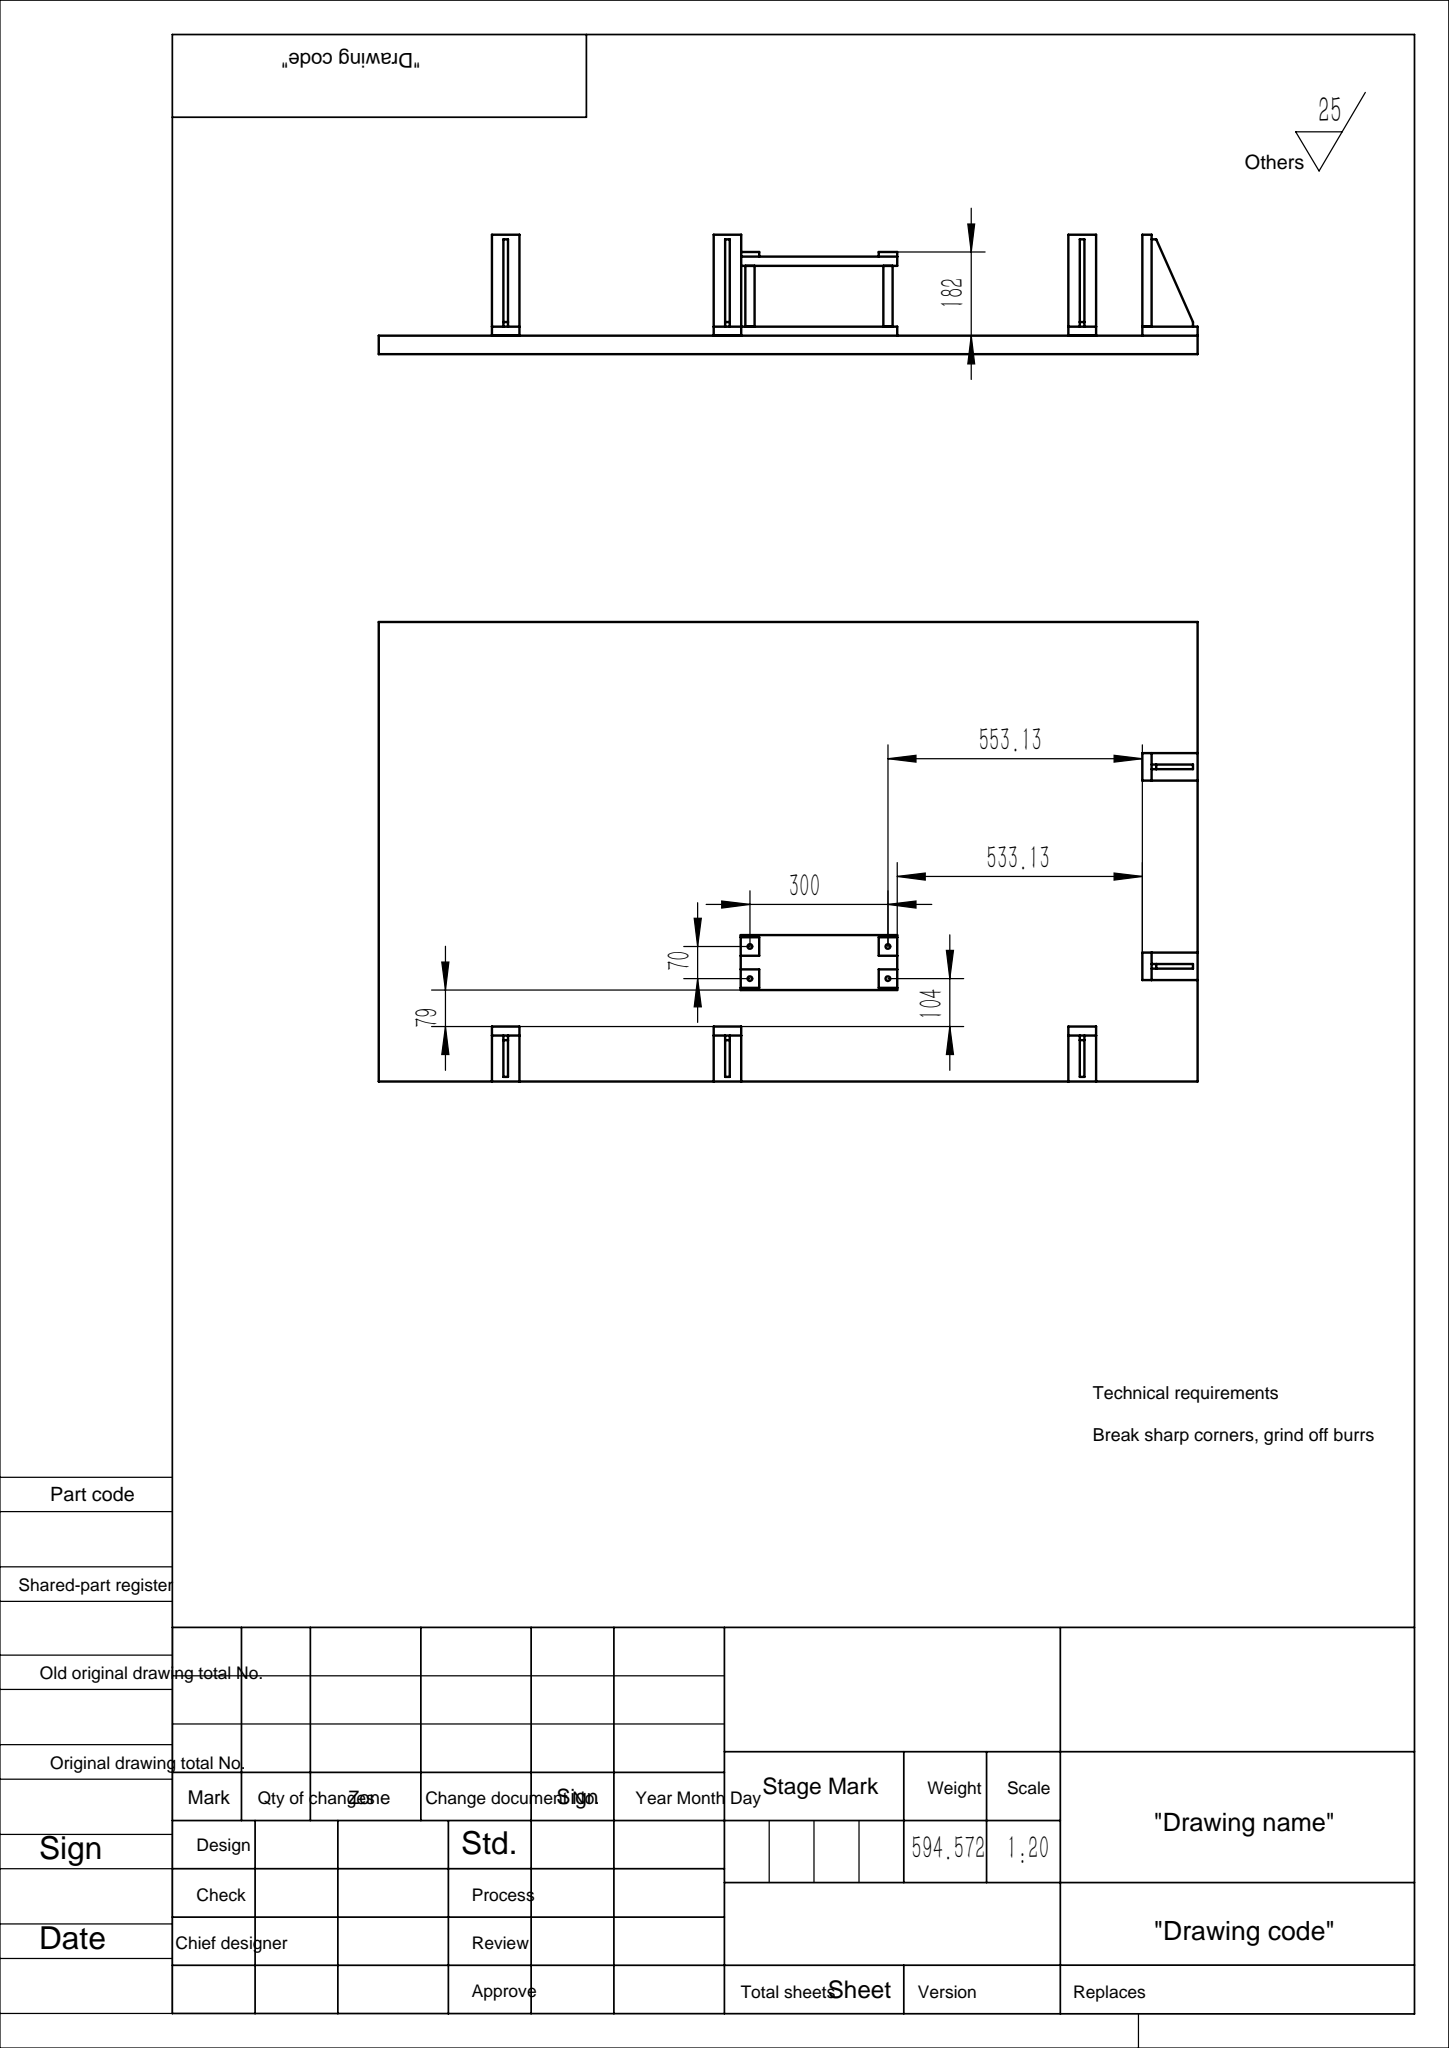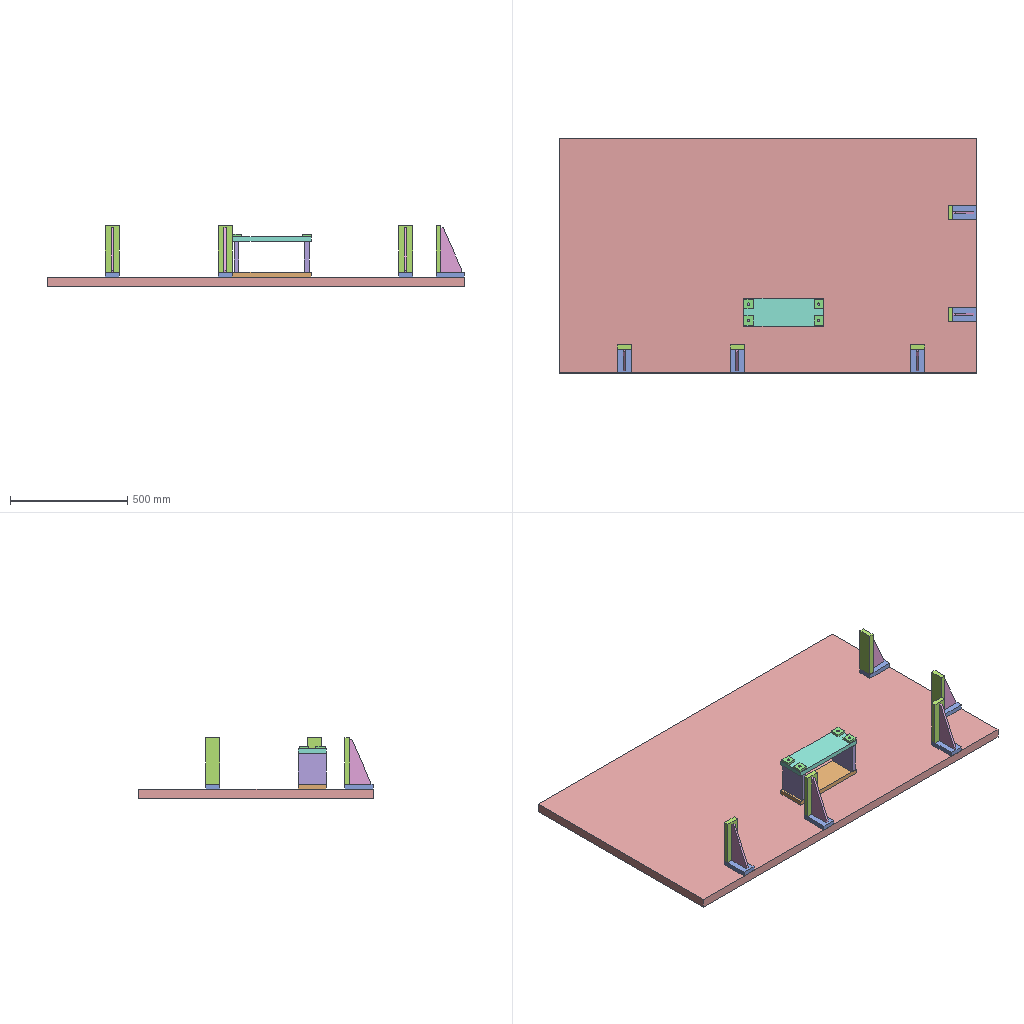Assembly | SolidWorks | 10 different items | 30 placed | box 1780 x 1000 x 260 mm
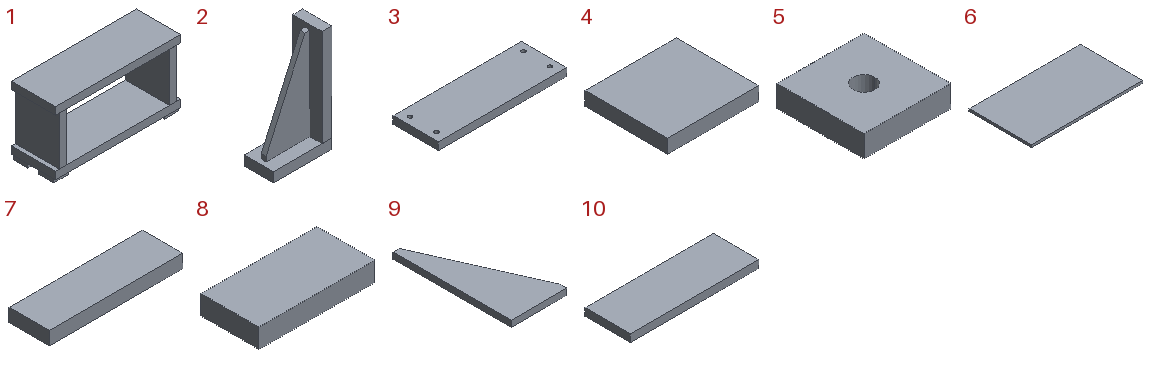Parts list (item | name | quantity | parent item | size | volume | features):
1 | (subassembly) | x1 | - | 340 x 120 x 182 mm | 2320175 mm3 | features CompositeCurve 1
2 | (subassembly) | x5 | - | 120 x 60 x 220 mm | 483000 mm3 | -
3 | - | x1 | in 1 | 340 x 120 x 20 mm | 809717 mm3 | features Extrusion 1
4 | - | x2 | in 1 | 132 x 120 x 20 mm | 316800 mm3 | features Extrusion 1
5 | - | x4 | in 1 | 40 x 40 x 10 mm | 15215 mm3 | features Extrusion 1
6 | - | x1 | - | 1780 x 1000 x 40 mm | 71200000 mm3 | features Extrusion 1
7 | - | x5 | in 2 | 200 x 60 x 20 mm | 240000 mm3 | features Extrusion 1
8 | - | x5 | in 2 | 120 x 60 x 20 mm | 144000 mm3 | features Extrusion 1
9 | - | x5 | in 2 | 90 x 190 x 10 mm | 99000 mm3 | features Extrusion 1
10 | - | x1 | in 1 | 340 x 120 x 20 mm | 816000 mm3 | features Extrusion 1
Mates (type | each side: item.copy, entity, surface, feature):
In the top assembly
DistanceDim | assembly face | 6.1 face plane Boss-Extrude1
Coincident | 6.1 face plane Boss-Extrude1 | 8.1 face plane Boss-Extrude1 | 2 times
Coincident | 7.1 face plane Boss-Extrude1 | 7.2 face plane Boss-Extrude1
Coincident | 7.1 face plane Boss-Extrude1 | 7.3 face plane Boss-Extrude1
Coincident | 7.1 face plane Boss-Extrude1 | 7.4 face plane Boss-Extrude1
Coincident | 7.1 face plane Boss-Extrude1 | 7.5 face plane Boss-Extrude1
Coincident | 6.1 face plane Boss-Extrude1 | 8.2 face plane Boss-Extrude1
Coincident | 6.1 face plane Boss-Extrude1 | 8.3 face plane Boss-Extrude1
Coincident | 6.1 face plane Boss-Extrude1 | 8.4 face plane Boss-Extrude1
Coincident | 6.1 face plane Boss-Extrude1 | 8.5 face plane Boss-Extrude1
Coincident | assembly face | 7.5 face plane Boss-Extrude1
Tangent | assembly face | 8.5 face plane Boss-Extrude1
Coincident | 6.1 face plane Boss-Extrude1 | 10.1 face plane Boss-Extrude1
Concentric | assembly face | 5.1 face cylinder Boss-Extrude1
Concentric | assembly face | 5.2 face cylinder Boss-Extrude1
Coincident | assembly face | 7.1 face plane Boss-Extrude1
In subassembly 2
Coincident | 8.6 face plane Boss-Extrude1 | 7.6 face plane Boss-Extrude1 | 3 times
Coincident | 7.6 face plane Boss-Extrude1 | 9.1 face plane Boss-Extrude1
Coincident | 8.6 face plane Boss-Extrude1 | 9.1 face plane Boss-Extrude1
DistanceDim | 9.1 face plane Boss-Extrude1 | 8.6 face plane Boss-Extrude1
In subassembly 1
Coincident | 3.1 face plane Boss-Extrude1 | 10.2 face plane Boss-Extrude1 | 2 times
DistanceDim | 10.2 face plane Boss-Extrude1 | 3.1 face plane Boss-Extrude1
Coincident | 3.1 face plane Boss-Extrude1 | 4.1 face plane Boss-Extrude1 | 2 times
DistanceDim | 4.1 face plane Boss-Extrude1 | 3.1 face plane Boss-Extrude1
Coincident | 3.1 face plane Boss-Extrude1 | 4.2 face plane Boss-Extrude1 | 2 times
DistanceDim | 4.2 face plane Boss-Extrude1 | 3.1 face plane Boss-Extrude1
Coincident | 3.1 face plane Boss-Extrude1 | 5.3 face plane Boss-Extrude1
Concentric | 3.1 face cylinder Boss-Extrude1 | 5.3 face cylinder Boss-Extrude1
Parallel | 3.1 face plane Boss-Extrude1 | 5.3 face plane Boss-Extrude1
Coincident | 5.4 face plane Boss-Extrude1 | 5.3 face plane Boss-Extrude1
Concentric | 3.1 face cylinder Boss-Extrude1 | 5.4 face cylinder Boss-Extrude1
Coincident | 5.5 face plane Boss-Extrude1 | 5.3 face plane Boss-Extrude1
Coincident | 5.6 face plane Boss-Extrude1 | 5.5 face plane Boss-Extrude1
Coincident | 3.1 edge | 5.5 face cylinder Boss-Extrude1
Concentric | 3.1 face cylinder Boss-Extrude1 | 5.6 face cylinder Boss-Extrude1
Parallel | 3.1 face plane Boss-Extrude1 | 5.5 face plane Boss-Extrude1
Parallel | 3.1 face plane Boss-Extrude1 | 5.6 face plane Boss-Extrude1
Parallel | 3.1 face plane Boss-Extrude1 | 5.4 face plane Boss-Extrude1